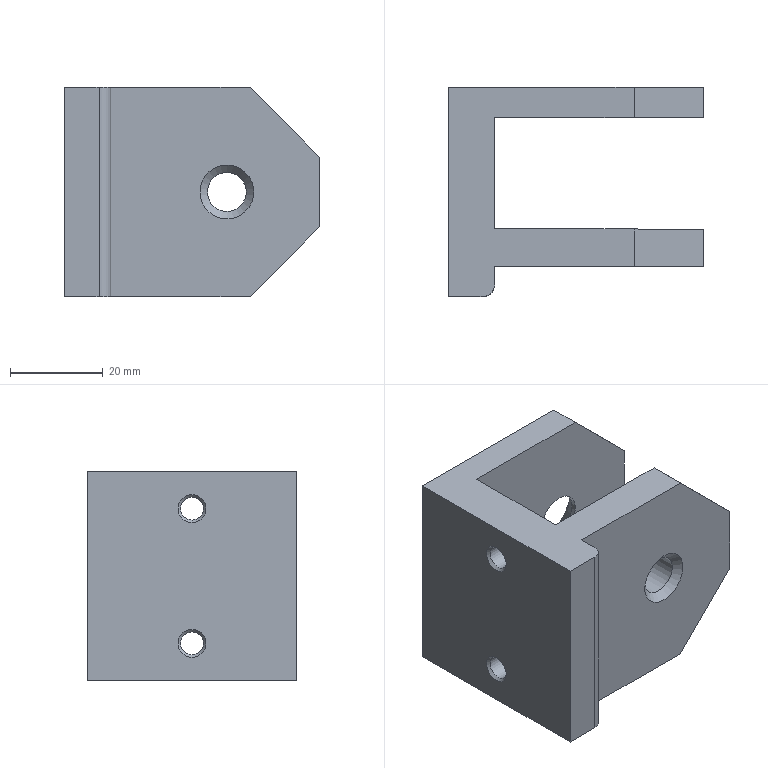Part | STEP file | HBLTBBN45_b | 1 solid | 26 faces | box 55 x 45 x 45 mm | volume 44256 mm3 | plane 16 | cylinder 5 | cone 5 | commonest cylinder face diameters 4.917 x2 5 x1 8.376 x1 10 x1
STEP:
#1=CARTESIAN_POINT('',(55.,45.,7.5));
#2=VERTEX_POINT('',#1);
#3=CARTESIAN_POINT('',(40.,45.,22.5));
#4=VERTEX_POINT('',#3);
#5=CARTESIAN_POINT('',(55.,45.,7.5));
#6=DIRECTION('',(-0.7071,0.,0.7071));
#7=VECTOR('',#6,1000.);
#8=LINE('',#5,#7);
#9=EDGE_CURVE('',#2,#4,#8,.T.);
#10=ORIENTED_EDGE('',*,*,#9,.F.);
#11=CARTESIAN_POINT('',(55.,45.,-7.5));
#12=VERTEX_POINT('',#11);
#13=CARTESIAN_POINT('',(55.,45.,22.5));
#14=DIRECTION('',(0.,0.,-1.));
#15=VECTOR('',#14,1000.);
#16=LINE('',#13,#15);
#17=EDGE_CURVE('',#2,#12,#16,.T.);
#18=ORIENTED_EDGE('',*,*,#17,.T.);
#19=CARTESIAN_POINT('',(40.,45.,-22.5));
#20=VERTEX_POINT('',#19);
#21=CARTESIAN_POINT('',(40.,45.,-22.5));
#22=DIRECTION('',(0.7071,0.,0.7071));
#23=VECTOR('',#22,1000.);
#24=LINE('',#21,#23);
#25=EDGE_CURVE('',#20,#12,#24,.T.);
#26=ORIENTED_EDGE('',*,*,#25,.F.);
#27=CARTESIAN_POINT('',(0.,45.,-22.5));
#28=VERTEX_POINT('',#27);
#29=CARTESIAN_POINT('',(55.,45.,-22.5));
#30=DIRECTION('',(-1.,0.,0.));
#31=VECTOR('',#30,1000.);
#32=LINE('',#29,#31);
#33=EDGE_CURVE('',#20,#28,#32,.T.);
#34=ORIENTED_EDGE('',*,*,#33,.T.);
#35=CARTESIAN_POINT('',(0.,45.,22.5));
#36=VERTEX_POINT('',#35);
#37=CARTESIAN_POINT('',(0.,45.,22.5));
#38=DIRECTION('',(0.,0.,-1.));
#39=VECTOR('',#38,1000.);
#40=LINE('',#37,#39);
#41=EDGE_CURVE('',#36,#28,#40,.T.);
#42=ORIENTED_EDGE('',*,*,#41,.F.);
#43=CARTESIAN_POINT('',(55.,45.,22.5));
#44=DIRECTION('',(-1.,0.,0.));
#45=VECTOR('',#44,1000.);
#46=LINE('',#43,#45);
#47=EDGE_CURVE('',#4,#36,#46,.T.);
#48=ORIENTED_EDGE('',*,*,#47,.F.);
#49=EDGE_LOOP('',(#10,#18,#26,#34,#42,#48));
#50=FACE_OUTER_BOUND('',#49,.T.);
#51=CARTESIAN_POINT('',(35.,45.,-10.5));
#52=VERTEX_POINT('',#51);
#53=CARTESIAN_POINT('',(35.,45.,0.));
#54=DIRECTION('',(0.,-1.,0.));
#55=DIRECTION('',(0.,0.,-1.));
#56=AXIS2_PLACEMENT_3D('',#53,#54,#55);
#57=CIRCLE('',#56,10.5);
#58=EDGE_CURVE('',#52,#52,#57,.T.);
#59=ORIENTED_EDGE('',*,*,#58,.T.);
#60=EDGE_LOOP('',(#59));
#61=FACE_BOUND('',#60,.T.);
#62=CARTESIAN_POINT('',(55.,45.,22.5));
#63=DIRECTION('',(0.,-1.,0.));
#64=DIRECTION('',(0.,0.,-1.));
#65=AXIS2_PLACEMENT_3D('',#62,#63,#64);
#66=PLANE('',#65);
#67=ADVANCED_FACE('',(#50,#61),#66,.F.);
#68=CARTESIAN_POINT('',(40.,6.5,22.5));
#69=VERTEX_POINT('',#68);
#70=CARTESIAN_POINT('',(55.,6.5,7.5));
#71=VERTEX_POINT('',#70);
#72=CARTESIAN_POINT('',(25.,6.5,37.5));
#73=DIRECTION('',(0.7071,0.,-0.7071));
#74=VECTOR('',#73,1000.);
#75=LINE('',#72,#74);
#76=EDGE_CURVE('',#69,#71,#75,.T.);
#77=ORIENTED_EDGE('',*,*,#76,.F.);
#78=CARTESIAN_POINT('',(10.,6.5,22.5));
#79=VERTEX_POINT('',#78);
#80=CARTESIAN_POINT('',(10.,6.5,22.5));
#81=DIRECTION('',(1.,0.,0.));
#82=VECTOR('',#81,1000.);
#83=LINE('',#80,#82);
#84=EDGE_CURVE('',#79,#69,#83,.T.);
#85=ORIENTED_EDGE('',*,*,#84,.F.);
#86=CARTESIAN_POINT('',(10.,6.5,-22.5));
#87=VERTEX_POINT('',#86);
#88=CARTESIAN_POINT('',(10.,6.5,22.5));
#89=DIRECTION('',(0.,0.,-1.));
#90=VECTOR('',#89,1000.);
#91=LINE('',#88,#90);
#92=EDGE_CURVE('',#79,#87,#91,.T.);
#93=ORIENTED_EDGE('',*,*,#92,.T.);
#94=CARTESIAN_POINT('',(40.,6.5,-22.5));
#95=VERTEX_POINT('',#94);
#96=CARTESIAN_POINT('',(10.,6.5,-22.5));
#97=DIRECTION('',(1.,0.,0.));
#98=VECTOR('',#97,1000.);
#99=LINE('',#96,#98);
#100=EDGE_CURVE('',#87,#95,#99,.T.);
#101=ORIENTED_EDGE('',*,*,#100,.T.);
#102=CARTESIAN_POINT('',(55.,6.5,-7.5));
#103=VERTEX_POINT('',#102);
#104=CARTESIAN_POINT('',(47.5,6.5,-15.));
#105=DIRECTION('',(-0.7071,0.,-0.7071));
#106=VECTOR('',#105,1000.);
#107=LINE('',#104,#106);
#108=EDGE_CURVE('',#103,#95,#107,.T.);
#109=ORIENTED_EDGE('',*,*,#108,.F.);
#110=CARTESIAN_POINT('',(55.,6.5,22.5));
#111=DIRECTION('',(0.,0.,-1.));
#112=VECTOR('',#111,1000.);
#113=LINE('',#110,#112);
#114=EDGE_CURVE('',#71,#103,#113,.T.);
#115=ORIENTED_EDGE('',*,*,#114,.F.);
#116=EDGE_LOOP('',(#77,#85,#93,#101,#109,#115));
#117=FACE_OUTER_BOUND('',#116,.T.);
#118=CARTESIAN_POINT('',(35.,6.5,-5.8));
#119=VERTEX_POINT('',#118);
#120=CARTESIAN_POINT('',(35.,6.5,5.8));
#121=VERTEX_POINT('',#120);
#122=CARTESIAN_POINT('',(35.,6.5,0.));
#123=DIRECTION('',(0.,-1.,0.));
#124=DIRECTION('',(0.,0.,-1.));
#125=AXIS2_PLACEMENT_3D('',#122,#123,#124);
#126=CIRCLE('',#125,5.8);
#127=EDGE_CURVE('',#119,#121,#126,.T.);
#128=ORIENTED_EDGE('',*,*,#127,.F.);
#129=CARTESIAN_POINT('',(35.,6.5,0.));
#130=DIRECTION('',(0.,-1.,0.));
#131=DIRECTION('',(0.,0.,-1.));
#132=AXIS2_PLACEMENT_3D('',#129,#130,#131);
#133=CIRCLE('',#132,5.8);
#134=EDGE_CURVE('',#121,#119,#133,.T.);
#135=ORIENTED_EDGE('',*,*,#134,.F.);
#136=EDGE_LOOP('',(#128,#135));
#137=FACE_BOUND('',#136,.T.);
#138=CARTESIAN_POINT('',(10.,6.5,22.5));
#139=DIRECTION('',(0.,1.,0.));
#140=DIRECTION('',(-1.,0.,0.));
#141=AXIS2_PLACEMENT_3D('',#138,#139,#140);
#142=PLANE('',#141);
#143=ADVANCED_FACE('',(#117,#137),#142,.F.);
#144=CARTESIAN_POINT('',(55.,14.5,7.5));
#145=VERTEX_POINT('',#144);
#146=CARTESIAN_POINT('',(55.,45.,7.5));
#147=DIRECTION('',(0.,-1.,0.));
#148=VECTOR('',#147,1000.);
#149=LINE('',#146,#148);
#150=EDGE_CURVE('',#145,#71,#149,.T.);
#151=ORIENTED_EDGE('',*,*,#150,.T.);
#152=ORIENTED_EDGE('',*,*,#114,.T.);
#153=CARTESIAN_POINT('',(55.,14.5,-7.5));
#154=VERTEX_POINT('',#153);
#155=CARTESIAN_POINT('',(55.,45.,-7.5));
#156=DIRECTION('',(0.,-1.,0.));
#157=VECTOR('',#156,1000.);
#158=LINE('',#155,#157);
#159=EDGE_CURVE('',#154,#103,#158,.T.);
#160=ORIENTED_EDGE('',*,*,#159,.F.);
#161=CARTESIAN_POINT('',(55.,14.5,22.5));
#162=DIRECTION('',(0.,0.,-1.));
#163=VECTOR('',#162,1000.);
#164=LINE('',#161,#163);
#165=EDGE_CURVE('',#145,#154,#164,.T.);
#166=ORIENTED_EDGE('',*,*,#165,.F.);
#167=EDGE_LOOP('',(#151,#152,#160,#166));
#168=FACE_OUTER_BOUND('',#167,.T.);
#169=CARTESIAN_POINT('',(55.,6.5,22.5));
#170=DIRECTION('',(-1.,0.,0.));
#171=DIRECTION('',(0.,0.,1.));
#172=AXIS2_PLACEMENT_3D('',#169,#170,#171);
#173=PLANE('',#172);
#174=ADVANCED_FACE('',(#168),#173,.F.);
#175=CARTESIAN_POINT('',(40.,14.5,22.5));
#176=VERTEX_POINT('',#175);
#177=CARTESIAN_POINT('',(47.5,14.5,15.));
#178=DIRECTION('',(-0.7071,0.,0.7071));
#179=VECTOR('',#178,1000.);
#180=LINE('',#177,#179);
#181=EDGE_CURVE('',#145,#176,#180,.T.);
#182=ORIENTED_EDGE('',*,*,#181,.F.);
#183=ORIENTED_EDGE('',*,*,#165,.T.);
#184=CARTESIAN_POINT('',(40.,14.5,-22.5));
#185=VERTEX_POINT('',#184);
#186=CARTESIAN_POINT('',(70.,14.5,7.5));
#187=DIRECTION('',(0.7071,0.,0.7071));
#188=VECTOR('',#187,1000.);
#189=LINE('',#186,#188);
#190=EDGE_CURVE('',#185,#154,#189,.T.);
#191=ORIENTED_EDGE('',*,*,#190,.F.);
#192=CARTESIAN_POINT('',(10.,14.5,-22.5));
#193=VERTEX_POINT('',#192);
#194=CARTESIAN_POINT('',(55.,14.5,-22.5));
#195=DIRECTION('',(-1.,0.,0.));
#196=VECTOR('',#195,1000.);
#197=LINE('',#194,#196);
#198=EDGE_CURVE('',#185,#193,#197,.T.);
#199=ORIENTED_EDGE('',*,*,#198,.T.);
#200=CARTESIAN_POINT('',(10.,14.5,22.5));
#201=VERTEX_POINT('',#200);
#202=CARTESIAN_POINT('',(10.,14.5,22.5));
#203=DIRECTION('',(0.,0.,-1.));
#204=VECTOR('',#203,1000.);
#205=LINE('',#202,#204);
#206=EDGE_CURVE('',#201,#193,#205,.T.);
#207=ORIENTED_EDGE('',*,*,#206,.F.);
#208=CARTESIAN_POINT('',(55.,14.5,22.5));
#209=DIRECTION('',(-1.,0.,0.));
#210=VECTOR('',#209,1000.);
#211=LINE('',#208,#210);
#212=EDGE_CURVE('',#176,#201,#211,.T.);
#213=ORIENTED_EDGE('',*,*,#212,.F.);
#214=EDGE_LOOP('',(#182,#183,#191,#199,#207,#213));
#215=FACE_OUTER_BOUND('',#214,.T.);
#216=CARTESIAN_POINT('',(35.,14.5,-5.));
#217=VERTEX_POINT('',#216);
#218=CARTESIAN_POINT('',(35.,14.5,0.));
#219=DIRECTION('',(0.,-1.,0.));
#220=DIRECTION('',(0.,0.,-1.));
#221=AXIS2_PLACEMENT_3D('',#218,#219,#220);
#222=CIRCLE('',#221,5.);
#223=EDGE_CURVE('',#217,#217,#222,.T.);
#224=ORIENTED_EDGE('',*,*,#223,.T.);
#225=EDGE_LOOP('',(#224));
#226=FACE_BOUND('',#225,.T.);
#227=CARTESIAN_POINT('',(55.,14.5,22.5));
#228=DIRECTION('',(0.,-1.,0.));
#229=DIRECTION('',(0.,0.,-1.));
#230=AXIS2_PLACEMENT_3D('',#227,#228,#229);
#231=PLANE('',#230);
#232=ADVANCED_FACE('',(#215,#226),#231,.F.);
#233=CARTESIAN_POINT('',(40.,38.5,22.5));
#234=VERTEX_POINT('',#233);
#235=CARTESIAN_POINT('',(55.,38.5,7.5));
#236=VERTEX_POINT('',#235);
#237=CARTESIAN_POINT('',(25.,38.5,37.5));
#238=DIRECTION('',(0.7071,0.,-0.7071));
#239=VECTOR('',#238,1000.);
#240=LINE('',#237,#239);
#241=EDGE_CURVE('',#234,#236,#240,.T.);
#242=ORIENTED_EDGE('',*,*,#241,.F.);
#243=CARTESIAN_POINT('',(10.,38.5,22.5));
#244=VERTEX_POINT('',#243);
#245=CARTESIAN_POINT('',(10.,38.5,22.5));
#246=DIRECTION('',(1.,0.,0.));
#247=VECTOR('',#246,1000.);
#248=LINE('',#245,#247);
#249=EDGE_CURVE('',#244,#234,#248,.T.);
#250=ORIENTED_EDGE('',*,*,#249,.F.);
#251=CARTESIAN_POINT('',(10.,38.5,-22.5));
#252=VERTEX_POINT('',#251);
#253=CARTESIAN_POINT('',(10.,38.5,22.5));
#254=DIRECTION('',(0.,0.,-1.));
#255=VECTOR('',#254,1000.);
#256=LINE('',#253,#255);
#257=EDGE_CURVE('',#244,#252,#256,.T.);
#258=ORIENTED_EDGE('',*,*,#257,.T.);
#259=CARTESIAN_POINT('',(40.,38.5,-22.5));
#260=VERTEX_POINT('',#259);
#261=CARTESIAN_POINT('',(10.,38.5,-22.5));
#262=DIRECTION('',(1.,0.,0.));
#263=VECTOR('',#262,1000.);
#264=LINE('',#261,#263);
#265=EDGE_CURVE('',#252,#260,#264,.T.);
#266=ORIENTED_EDGE('',*,*,#265,.T.);
#267=CARTESIAN_POINT('',(55.,38.5,-7.5));
#268=VERTEX_POINT('',#267);
#269=CARTESIAN_POINT('',(47.5,38.5,-15.));
#270=DIRECTION('',(-0.7071,0.,-0.7071));
#271=VECTOR('',#270,1000.);
#272=LINE('',#269,#271);
#273=EDGE_CURVE('',#268,#260,#272,.T.);
#274=ORIENTED_EDGE('',*,*,#273,.F.);
#275=CARTESIAN_POINT('',(55.,38.5,22.5));
#276=DIRECTION('',(0.,0.,-1.));
#277=VECTOR('',#276,1000.);
#278=LINE('',#275,#277);
#279=EDGE_CURVE('',#236,#268,#278,.T.);
#280=ORIENTED_EDGE('',*,*,#279,.F.);
#281=EDGE_LOOP('',(#242,#250,#258,#266,#274,#280));
#282=FACE_OUTER_BOUND('',#281,.T.);
#283=CARTESIAN_POINT('',(35.,38.5,-5.));
#284=VERTEX_POINT('',#283);
#285=CARTESIAN_POINT('',(35.,38.5,5.));
#286=VERTEX_POINT('',#285);
#287=CARTESIAN_POINT('',(35.,38.5,0.));
#288=DIRECTION('',(0.,-1.,0.));
#289=DIRECTION('',(0.,0.,-1.));
#290=AXIS2_PLACEMENT_3D('',#287,#288,#289);
#291=CIRCLE('',#290,5.);
#292=EDGE_CURVE('',#284,#286,#291,.T.);
#293=ORIENTED_EDGE('',*,*,#292,.F.);
#294=CARTESIAN_POINT('',(35.,38.5,0.));
#295=DIRECTION('',(0.,-1.,0.));
#296=DIRECTION('',(0.,0.,-1.));
#297=AXIS2_PLACEMENT_3D('',#294,#295,#296);
#298=CIRCLE('',#297,5.);
#299=EDGE_CURVE('',#286,#284,#298,.T.);
#300=ORIENTED_EDGE('',*,*,#299,.F.);
#301=EDGE_LOOP('',(#293,#300));
#302=FACE_BOUND('',#301,.T.);
#303=CARTESIAN_POINT('',(10.,38.5,22.5));
#304=DIRECTION('',(0.,1.,0.));
#305=DIRECTION('',(0.,0.,1.));
#306=AXIS2_PLACEMENT_3D('',#303,#304,#305);
#307=PLANE('',#306);
#308=ADVANCED_FACE('',(#282,#302),#307,.F.);
#309=CARTESIAN_POINT('',(55.,45.,7.5));
#310=DIRECTION('',(0.,-1.,0.));
#311=VECTOR('',#310,1000.);
#312=LINE('',#309,#311);
#313=EDGE_CURVE('',#2,#236,#312,.T.);
#314=ORIENTED_EDGE('',*,*,#313,.T.);
#315=ORIENTED_EDGE('',*,*,#279,.T.);
#316=CARTESIAN_POINT('',(55.,45.,-7.5));
#317=DIRECTION('',(0.,-1.,0.));
#318=VECTOR('',#317,1000.);
#319=LINE('',#316,#318);
#320=EDGE_CURVE('',#12,#268,#319,.T.);
#321=ORIENTED_EDGE('',*,*,#320,.F.);
#322=ORIENTED_EDGE('',*,*,#17,.F.);
#323=EDGE_LOOP('',(#314,#315,#321,#322));
#324=FACE_OUTER_BOUND('',#323,.T.);
#325=CARTESIAN_POINT('',(55.,38.5,22.5));
#326=DIRECTION('',(-1.,0.,0.));
#327=DIRECTION('',(0.,0.,1.));
#328=AXIS2_PLACEMENT_3D('',#325,#326,#327);
#329=PLANE('',#328);
#330=ADVANCED_FACE('',(#324),#329,.F.);
#331=ORIENTED_EDGE('',*,*,#84,.T.);
#332=CARTESIAN_POINT('',(40.,2.5,22.5));
#333=DIRECTION('',(0.,1.,0.));
#334=VECTOR('',#333,1000.);
#335=LINE('',#332,#334);
#336=EDGE_CURVE('',#69,#176,#335,.T.);
#337=ORIENTED_EDGE('',*,*,#336,.T.);
#338=ORIENTED_EDGE('',*,*,#212,.T.);
#339=CARTESIAN_POINT('',(10.,14.5,22.5));
#340=DIRECTION('',(0.,1.,0.));
#341=VECTOR('',#340,1000.);
#342=LINE('',#339,#341);
#343=EDGE_CURVE('',#201,#244,#342,.T.);
#344=ORIENTED_EDGE('',*,*,#343,.T.);
#345=ORIENTED_EDGE('',*,*,#249,.T.);
#346=CARTESIAN_POINT('',(40.,45.,22.5));
#347=DIRECTION('',(0.,-1.,0.));
#348=VECTOR('',#347,1000.);
#349=LINE('',#346,#348);
#350=EDGE_CURVE('',#4,#234,#349,.T.);
#351=ORIENTED_EDGE('',*,*,#350,.F.);
#352=ORIENTED_EDGE('',*,*,#47,.T.);
#353=CARTESIAN_POINT('',(0.,0.,22.5));
#354=VERTEX_POINT('',#353);
#355=CARTESIAN_POINT('',(0.,45.,22.5));
#356=DIRECTION('',(0.,-1.,0.));
#357=VECTOR('',#356,1000.);
#358=LINE('',#355,#357);
#359=EDGE_CURVE('',#36,#354,#358,.T.);
#360=ORIENTED_EDGE('',*,*,#359,.T.);
#361=CARTESIAN_POINT('',(7.5,0.,22.5));
#362=VERTEX_POINT('',#361);
#363=CARTESIAN_POINT('',(0.,0.,22.5));
#364=DIRECTION('',(1.,0.,0.));
#365=VECTOR('',#364,1000.);
#366=LINE('',#363,#365);
#367=EDGE_CURVE('',#354,#362,#366,.T.);
#368=ORIENTED_EDGE('',*,*,#367,.T.);
#369=CARTESIAN_POINT('',(10.,2.5,22.5));
#370=VERTEX_POINT('',#369);
#371=CARTESIAN_POINT('',(7.5,2.5,22.5));
#372=DIRECTION('',(0.,0.,1.));
#373=DIRECTION('',(1.,0.,0.));
#374=AXIS2_PLACEMENT_3D('',#371,#372,#373);
#375=CIRCLE('',#374,2.5);
#376=EDGE_CURVE('',#362,#370,#375,.T.);
#377=ORIENTED_EDGE('',*,*,#376,.T.);
#378=CARTESIAN_POINT('',(10.,2.5,22.5));
#379=DIRECTION('',(0.,1.,0.));
#380=VECTOR('',#379,1000.);
#381=LINE('',#378,#380);
#382=EDGE_CURVE('',#370,#79,#381,.T.);
#383=ORIENTED_EDGE('',*,*,#382,.T.);
#384=EDGE_LOOP('',(#331,#337,#338,#344,#345,#351,#352,#360,#368,#377,#383));
#385=FACE_OUTER_BOUND('',#384,.T.);
#386=CARTESIAN_POINT('',(7.5,2.5,22.5));
#387=DIRECTION('',(0.,0.,1.));
#388=DIRECTION('',(1.,0.,0.));
#389=AXIS2_PLACEMENT_3D('',#386,#387,#388);
#390=PLANE('',#389);
#391=ADVANCED_FACE('',(#385),#390,.T.);
#392=CARTESIAN_POINT('',(40.,2.5,-22.5));
#393=DIRECTION('',(0.,1.,0.));
#394=VECTOR('',#393,1000.);
#395=LINE('',#392,#394);
#396=EDGE_CURVE('',#95,#185,#395,.T.);
#397=ORIENTED_EDGE('',*,*,#396,.F.);
#398=ORIENTED_EDGE('',*,*,#100,.F.);
#399=CARTESIAN_POINT('',(10.,2.5,-22.5));
#400=VERTEX_POINT('',#399);
#401=CARTESIAN_POINT('',(10.,2.5,-22.5));
#402=DIRECTION('',(0.,1.,0.));
#403=VECTOR('',#402,1000.);
#404=LINE('',#401,#403);
#405=EDGE_CURVE('',#400,#87,#404,.T.);
#406=ORIENTED_EDGE('',*,*,#405,.F.);
#407=CARTESIAN_POINT('',(7.5,0.,-22.5));
#408=VERTEX_POINT('',#407);
#409=CARTESIAN_POINT('',(7.5,2.5,-22.5));
#410=DIRECTION('',(0.,0.,1.));
#411=DIRECTION('',(1.,0.,0.));
#412=AXIS2_PLACEMENT_3D('',#409,#410,#411);
#413=CIRCLE('',#412,2.5);
#414=EDGE_CURVE('',#408,#400,#413,.T.);
#415=ORIENTED_EDGE('',*,*,#414,.F.);
#416=CARTESIAN_POINT('',(0.,0.,-22.5));
#417=VERTEX_POINT('',#416);
#418=CARTESIAN_POINT('',(0.,0.,-22.5));
#419=DIRECTION('',(1.,0.,0.));
#420=VECTOR('',#419,1000.);
#421=LINE('',#418,#420);
#422=EDGE_CURVE('',#417,#408,#421,.T.);
#423=ORIENTED_EDGE('',*,*,#422,.F.);
#424=CARTESIAN_POINT('',(0.,45.,-22.5));
#425=DIRECTION('',(0.,-1.,0.));
#426=VECTOR('',#425,1000.);
#427=LINE('',#424,#426);
#428=EDGE_CURVE('',#28,#417,#427,.T.);
#429=ORIENTED_EDGE('',*,*,#428,.F.);
#430=ORIENTED_EDGE('',*,*,#33,.F.);
#431=CARTESIAN_POINT('',(40.,45.,-22.5));
#432=DIRECTION('',(0.,-1.,0.));
#433=VECTOR('',#432,1000.);
#434=LINE('',#431,#433);
#435=EDGE_CURVE('',#20,#260,#434,.T.);
#436=ORIENTED_EDGE('',*,*,#435,.T.);
#437=ORIENTED_EDGE('',*,*,#265,.F.);
#438=CARTESIAN_POINT('',(10.,14.5,-22.5));
#439=DIRECTION('',(0.,1.,0.));
#440=VECTOR('',#439,1000.);
#441=LINE('',#438,#440);
#442=EDGE_CURVE('',#193,#252,#441,.T.);
#443=ORIENTED_EDGE('',*,*,#442,.F.);
#444=ORIENTED_EDGE('',*,*,#198,.F.);
#445=EDGE_LOOP('',(#397,#398,#406,#415,#423,#429,#430,#436,#437,#443,#444));
#446=FACE_OUTER_BOUND('',#445,.T.);
#447=CARTESIAN_POINT('',(7.5,2.5,-22.5));
#448=DIRECTION('',(0.,0.,1.));
#449=DIRECTION('',(1.,0.,0.));
#450=AXIS2_PLACEMENT_3D('',#447,#448,#449);
#451=PLANE('',#450);
#452=ADVANCED_FACE('',(#446),#451,.F.);
#453=ORIENTED_EDGE('',*,*,#428,.T.);
#454=CARTESIAN_POINT('',(0.,0.,22.5));
#455=DIRECTION('',(0.,0.,-1.));
#456=VECTOR('',#455,1000.);
#457=LINE('',#454,#456);
#458=EDGE_CURVE('',#354,#417,#457,.T.);
#459=ORIENTED_EDGE('',*,*,#458,.F.);
#460=ORIENTED_EDGE('',*,*,#359,.F.);
#461=ORIENTED_EDGE('',*,*,#41,.T.);
#462=EDGE_LOOP('',(#453,#459,#460,#461));
#463=FACE_OUTER_BOUND('',#462,.T.);
#464=CARTESIAN_POINT('',(0.,22.5,-17.5));
#465=VERTEX_POINT('',#464);
#466=CARTESIAN_POINT('',(0.,22.5,-14.5));
#467=DIRECTION('',(1.,0.,0.));
#468=DIRECTION('',(0.,0.,-1.));
#469=AXIS2_PLACEMENT_3D('',#466,#467,#468);
#470=CIRCLE('',#469,3.);
#471=EDGE_CURVE('',#465,#465,#470,.T.);
#472=ORIENTED_EDGE('',*,*,#471,.T.);
#473=EDGE_LOOP('',(#472));
#474=FACE_BOUND('',#473,.T.);
#475=CARTESIAN_POINT('',(0.,22.5,11.5));
#476=VERTEX_POINT('',#475);
#477=CARTESIAN_POINT('',(0.,22.5,14.5));
#478=DIRECTION('',(1.,0.,0.));
#479=DIRECTION('',(0.,0.,-1.));
#480=AXIS2_PLACEMENT_3D('',#477,#478,#479);
#481=CIRCLE('',#480,3.);
#482=EDGE_CURVE('',#476,#476,#481,.T.);
#483=ORIENTED_EDGE('',*,*,#482,.T.);
#484=EDGE_LOOP('',(#483));
#485=FACE_BOUND('',#484,.T.);
#486=CARTESIAN_POINT('',(0.,45.,22.5));
#487=DIRECTION('',(1.,0.,0.));
#488=DIRECTION('',(0.,0.,-1.));
#489=AXIS2_PLACEMENT_3D('',#486,#487,#488);
#490=PLANE('',#489);
#491=ADVANCED_FACE('',(#463,#474,#485),#490,.F.);
#492=ORIENTED_EDGE('',*,*,#422,.T.);
#493=CARTESIAN_POINT('',(7.5,0.,22.5));
#494=DIRECTION('',(0.,0.,-1.));
#495=VECTOR('',#494,1000.);
#496=LINE('',#493,#495);
#497=EDGE_CURVE('',#362,#408,#496,.T.);
#498=ORIENTED_EDGE('',*,*,#497,.F.);
#499=ORIENTED_EDGE('',*,*,#367,.F.);
#500=ORIENTED_EDGE('',*,*,#458,.T.);
#501=EDGE_LOOP('',(#492,#498,#499,#500));
#502=FACE_OUTER_BOUND('',#501,.T.);
#503=CARTESIAN_POINT('',(0.,0.,22.5));
#504=DIRECTION('',(0.,1.,0.));
#505=DIRECTION('',(0.,0.,1.));
#506=AXIS2_PLACEMENT_3D('',#503,#504,#505);
#507=PLANE('',#506);
#508=ADVANCED_FACE('',(#502),#507,.F.);
#509=ORIENTED_EDGE('',*,*,#414,.T.);
#510=CARTESIAN_POINT('',(10.,2.5,22.5));
#511=DIRECTION('',(0.,0.,-1.));
#512=VECTOR('',#511,1000.);
#513=LINE('',#510,#512);
#514=EDGE_CURVE('',#370,#400,#513,.T.);
#515=ORIENTED_EDGE('',*,*,#514,.F.);
#516=ORIENTED_EDGE('',*,*,#376,.F.);
#517=ORIENTED_EDGE('',*,*,#497,.T.);
#518=EDGE_LOOP('',(#509,#515,#516,#517));
#519=FACE_OUTER_BOUND('',#518,.T.);
#520=CARTESIAN_POINT('',(7.5,2.5,22.5));
#521=DIRECTION('',(0.,0.,-1.));
#522=DIRECTION('',(-1.,0.,0.));
#523=AXIS2_PLACEMENT_3D('',#520,#521,#522);
#524=CYLINDRICAL_SURFACE('',#523,2.5);
#525=ADVANCED_FACE('',(#519),#524,.T.);
#526=ORIENTED_EDGE('',*,*,#405,.T.);
#527=ORIENTED_EDGE('',*,*,#92,.F.);
#528=ORIENTED_EDGE('',*,*,#382,.F.);
#529=ORIENTED_EDGE('',*,*,#514,.T.);
#530=EDGE_LOOP('',(#526,#527,#528,#529));
#531=FACE_OUTER_BOUND('',#530,.T.);
#532=CARTESIAN_POINT('',(10.,2.5,22.5));
#533=DIRECTION('',(-1.,0.,0.));
#534=DIRECTION('',(0.,0.,1.));
#535=AXIS2_PLACEMENT_3D('',#532,#533,#534);
#536=PLANE('',#535);
#537=ADVANCED_FACE('',(#531),#536,.F.);
#538=ORIENTED_EDGE('',*,*,#442,.T.);
#539=ORIENTED_EDGE('',*,*,#257,.F.);
#540=ORIENTED_EDGE('',*,*,#343,.F.);
#541=ORIENTED_EDGE('',*,*,#206,.T.);
#542=EDGE_LOOP('',(#538,#539,#540,#541));
#543=FACE_OUTER_BOUND('',#542,.T.);
#544=CARTESIAN_POINT('',(10.,22.5,-16.959));
#545=VERTEX_POINT('',#544);
#546=CARTESIAN_POINT('',(10.,22.5,-12.041));
#547=VERTEX_POINT('',#546);
#548=CARTESIAN_POINT('',(10.,22.5,-14.5));
#549=DIRECTION('',(1.,0.,0.));
#550=DIRECTION('',(0.,0.,-1.));
#551=AXIS2_PLACEMENT_3D('',#548,#549,#550);
#552=CIRCLE('',#551,2.458);
#553=EDGE_CURVE('',#545,#547,#552,.T.);
#554=ORIENTED_EDGE('',*,*,#553,.F.);
#555=CARTESIAN_POINT('',(10.,22.5,-14.5));
#556=DIRECTION('',(1.,0.,0.));
#557=DIRECTION('',(0.,0.,-1.));
#558=AXIS2_PLACEMENT_3D('',#555,#556,#557);
#559=CIRCLE('',#558,2.458);
#560=EDGE_CURVE('',#547,#545,#559,.T.);
#561=ORIENTED_EDGE('',*,*,#560,.F.);
#562=EDGE_LOOP('',(#554,#561));
#563=FACE_BOUND('',#562,.T.);
#564=CARTESIAN_POINT('',(10.,22.5,12.041));
#565=VERTEX_POINT('',#564);
#566=CARTESIAN_POINT('',(10.,22.5,16.959));
#567=VERTEX_POINT('',#566);
#568=CARTESIAN_POINT('',(10.,22.5,14.5));
#569=DIRECTION('',(1.,0.,0.));
#570=DIRECTION('',(0.,0.,-1.));
#571=AXIS2_PLACEMENT_3D('',#568,#569,#570);
#572=CIRCLE('',#571,2.458);
#573=EDGE_CURVE('',#565,#567,#572,.T.);
#574=ORIENTED_EDGE('',*,*,#573,.F.);
#575=CARTESIAN_POINT('',(10.,22.5,14.5));
#576=DIRECTION('',(1.,0.,0.));
#577=DIRECTION('',(0.,0.,-1.));
#578=AXIS2_PLACEMENT_3D('',#575,#576,#577);
#579=CIRCLE('',#578,2.458);
#580=EDGE_CURVE('',#567,#565,#579,.T.);
#581=ORIENTED_EDGE('',*,*,#580,.F.);
#582=EDGE_LOOP('',(#574,#581));
#583=FACE_BOUND('',#582,.T.);
#584=CARTESIAN_POINT('',(10.,14.5,22.5));
#585=DIRECTION('',(-1.,0.,0.));
#586=DIRECTION('',(0.,0.,1.));
#587=AXIS2_PLACEMENT_3D('',#584,#585,#586);
#588=PLANE('',#587);
#589=ADVANCED_FACE('',(#543,#563,#583),#588,.F.);
#590=ORIENTED_EDGE('',*,*,#273,.T.);
#591=ORIENTED_EDGE('',*,*,#435,.F.);
#592=ORIENTED_EDGE('',*,*,#25,.T.);
#593=ORIENTED_EDGE('',*,*,#320,.T.);
#594=EDGE_LOOP('',(#590,#591,#592,#593));
#595=FACE_OUTER_BOUND('',#594,.T.);
#596=CARTESIAN_POINT('',(40.,45.,-22.5));
#597=DIRECTION('',(0.7071,0.,-0.7071));
#598=DIRECTION('',(-0.7071,0.,-0.7071));
#599=AXIS2_PLACEMENT_3D('',#596,#597,#598);
#600=PLANE('',#599);
#601=ADVANCED_FACE('',(#595),#600,.T.);
#602=ORIENTED_EDGE('',*,*,#108,.T.);
#603=ORIENTED_EDGE('',*,*,#396,.T.);
#604=ORIENTED_EDGE('',*,*,#190,.T.);
#605=ORIENTED_EDGE('',*,*,#159,.T.);
#606=EDGE_LOOP('',(#602,#603,#604,#605));
#607=FACE_OUTER_BOUND('',#606,.T.);
#608=CARTESIAN_POINT('',(40.,45.,-22.5));
#609=DIRECTION('',(0.7071,0.,-0.7071));
#610=DIRECTION('',(-0.7071,0.,-0.7071));
#611=AXIS2_PLACEMENT_3D('',#608,#609,#610);
#612=PLANE('',#611);
#613=ADVANCED_FACE('',(#607),#612,.T.);
#614=ORIENTED_EDGE('',*,*,#241,.T.);
#615=ORIENTED_EDGE('',*,*,#313,.F.);
#616=ORIENTED_EDGE('',*,*,#9,.T.);
#617=ORIENTED_EDGE('',*,*,#350,.T.);
#618=EDGE_LOOP('',(#614,#615,#616,#617));
#619=FACE_OUTER_BOUND('',#618,.T.);
#620=CARTESIAN_POINT('',(55.,45.,7.5));
#621=DIRECTION('',(0.7071,0.,0.7071));
#622=DIRECTION('',(0.7071,0.,-0.7071));
#623=AXIS2_PLACEMENT_3D('',#620,#621,#622);
#624=PLANE('',#623);
#625=ADVANCED_FACE('',(#619),#624,.T.);
#626=ORIENTED_EDGE('',*,*,#76,.T.);
#627=ORIENTED_EDGE('',*,*,#150,.F.);
#628=ORIENTED_EDGE('',*,*,#181,.T.);
#629=ORIENTED_EDGE('',*,*,#336,.F.);
#630=EDGE_LOOP('',(#626,#627,#628,#629));
#631=FACE_OUTER_BOUND('',#630,.T.);
#632=CARTESIAN_POINT('',(55.,45.,7.5));
#633=DIRECTION('',(0.7071,0.,0.7071));
#634=DIRECTION('',(0.7071,0.,-0.7071));
#635=AXIS2_PLACEMENT_3D('',#632,#633,#634);
#636=PLANE('',#635);
#637=ADVANCED_FACE('',(#631),#636,.T.);
#638=CARTESIAN_POINT('',(35.,13.688,-4.188));
#639=VERTEX_POINT('',#638);
#640=CARTESIAN_POINT('',(35.,13.688,4.188));
#641=VERTEX_POINT('',#640);
#642=CARTESIAN_POINT('',(35.,13.688,0.));
#643=DIRECTION('',(0.,-1.,0.));
#644=DIRECTION('',(0.,0.,-1.));
#645=AXIS2_PLACEMENT_3D('',#642,#643,#644);
#646=CIRCLE('',#645,4.188);
#647=EDGE_CURVE('',#639,#641,#646,.T.);
#648=ORIENTED_EDGE('',*,*,#647,.T.);
#649=CARTESIAN_POINT('',(35.,13.688,0.));
#650=DIRECTION('',(0.,-1.,0.));
#651=DIRECTION('',(0.,0.,-1.));
#652=AXIS2_PLACEMENT_3D('',#649,#650,#651);
#653=CIRCLE('',#652,4.188);
#654=EDGE_CURVE('',#641,#639,#653,.T.);
#655=ORIENTED_EDGE('',*,*,#654,.T.);
#656=CARTESIAN_POINT('',(35.,14.5,-5.));
#657=DIRECTION('',(0.,0.7071,-0.7071));
#658=VECTOR('',#657,5.);
#659=LINE('',#656,#658);
#660=EDGE_CURVE('',#639,#217,#659,.T.);
#661=ORIENTED_EDGE('',*,*,#660,.T.);
#662=ORIENTED_EDGE('',*,*,#223,.F.);
#663=ORIENTED_EDGE('',*,*,#660,.F.);
#664=EDGE_LOOP('',(#648,#655,#661,#662,#663));
#665=FACE_OUTER_BOUND('',#664,.T.);
#666=CARTESIAN_POINT('',(35.,14.5,0.));
#667=DIRECTION('',(0.,1.,0.));
#668=DIRECTION('',(0.,0.,1.));
#669=AXIS2_PLACEMENT_3D('',#666,#667,#668);
#670=CONICAL_SURFACE('',#669,5.,0.7854);
#671=ADVANCED_FACE('',(#665),#670,.F.);
#672=ORIENTED_EDGE('',*,*,#647,.F.);
#673=ORIENTED_EDGE('',*,*,#654,.F.);
#674=CARTESIAN_POINT('',(35.,8.112,4.188));
#675=VERTEX_POINT('',#674);
#676=CARTESIAN_POINT('',(35.,6.5,4.188));
#677=DIRECTION('',(0.,-1.,0.));
#678=VECTOR('',#677,4.188);
#679=LINE('',#676,#678);
#680=EDGE_CURVE('',#641,#675,#679,.T.);
#681=ORIENTED_EDGE('',*,*,#680,.T.);
#682=CARTESIAN_POINT('',(35.,8.112,-4.188));
#683=VERTEX_POINT('',#682);
#684=CARTESIAN_POINT('',(35.,8.112,0.));
#685=DIRECTION('',(0.,-1.,0.));
#686=DIRECTION('',(0.,0.,-1.));
#687=AXIS2_PLACEMENT_3D('',#684,#685,#686);
#688=CIRCLE('',#687,4.188);
#689=EDGE_CURVE('',#675,#683,#688,.T.);
#690=ORIENTED_EDGE('',*,*,#689,.T.);
#691=CARTESIAN_POINT('',(35.,8.112,0.));
#692=DIRECTION('',(0.,-1.,0.));
#693=DIRECTION('',(0.,0.,-1.));
#694=AXIS2_PLACEMENT_3D('',#691,#692,#693);
#695=CIRCLE('',#694,4.188);
#696=EDGE_CURVE('',#683,#675,#695,.T.);
#697=ORIENTED_EDGE('',*,*,#696,.T.);
#698=ORIENTED_EDGE('',*,*,#680,.F.);
#699=EDGE_LOOP('',(#672,#673,#681,#690,#697,#698));
#700=FACE_OUTER_BOUND('',#699,.T.);
#701=CARTESIAN_POINT('',(35.,6.5,0.));
#702=DIRECTION('',(0.,-1.,0.));
#703=DIRECTION('',(0.,0.,-1.));
#704=AXIS2_PLACEMENT_3D('',#701,#702,#703);
#705=CYLINDRICAL_SURFACE('',#704,4.188);
#706=ADVANCED_FACE('',(#700),#705,.F.);
#707=ORIENTED_EDGE('',*,*,#696,.F.);
#708=ORIENTED_EDGE('',*,*,#689,.F.);
#709=CARTESIAN_POINT('',(35.,8.112,4.188));
#710=DIRECTION('',(0.,-0.7071,0.7071));
#711=VECTOR('',#710,4.188);
#712=LINE('',#709,#711);
#713=EDGE_CURVE('',#675,#121,#712,.T.);
#714=ORIENTED_EDGE('',*,*,#713,.T.);
#715=ORIENTED_EDGE('',*,*,#134,.T.);
#716=ORIENTED_EDGE('',*,*,#127,.T.);
#717=ORIENTED_EDGE('',*,*,#713,.F.);
#718=EDGE_LOOP('',(#707,#708,#714,#715,#716,#717));
#719=FACE_OUTER_BOUND('',#718,.T.);
#720=CARTESIAN_POINT('',(35.,8.112,0.));
#721=DIRECTION('',(0.,-1.,0.));
#722=DIRECTION('',(0.,0.,-1.));
#723=AXIS2_PLACEMENT_3D('',#720,#721,#722);
#724=CONICAL_SURFACE('',#723,4.188,0.7854);
#725=ADVANCED_FACE('',(#719),#724,.F.);
#726=CARTESIAN_POINT('',(35.,39.5,-5.));
#727=VERTEX_POINT('',#726);
#728=CARTESIAN_POINT('',(35.,39.5,5.));
#729=VERTEX_POINT('',#728);
#730=CARTESIAN_POINT('',(35.,39.5,0.));
#731=DIRECTION('',(0.,-1.,0.));
#732=DIRECTION('',(0.,0.,-1.));
#733=AXIS2_PLACEMENT_3D('',#730,#731,#732);
#734=CIRCLE('',#733,5.);
#735=EDGE_CURVE('',#727,#729,#734,.T.);
#736=ORIENTED_EDGE('',*,*,#735,.T.);
#737=CARTESIAN_POINT('',(35.,39.5,0.));
#738=DIRECTION('',(0.,-1.,0.));
#739=DIRECTION('',(0.,0.,-1.));
#740=AXIS2_PLACEMENT_3D('',#737,#738,#739);
#741=CIRCLE('',#740,5.);
#742=EDGE_CURVE('',#729,#727,#741,.T.);
#743=ORIENTED_EDGE('',*,*,#742,.T.);
#744=CARTESIAN_POINT('',(35.,45.,-10.5));
#745=DIRECTION('',(0.,0.7071,-0.7071));
#746=VECTOR('',#745,10.5);
#747=LINE('',#744,#746);
#748=EDGE_CURVE('',#727,#52,#747,.T.);
#749=ORIENTED_EDGE('',*,*,#748,.T.);
#750=ORIENTED_EDGE('',*,*,#58,.F.);
#751=ORIENTED_EDGE('',*,*,#748,.F.);
#752=EDGE_LOOP('',(#736,#743,#749,#750,#751));
#753=FACE_OUTER_BOUND('',#752,.T.);
#754=CARTESIAN_POINT('',(35.,45.,0.));
#755=DIRECTION('',(0.,1.,0.));
#756=DIRECTION('',(0.,0.,1.));
#757=AXIS2_PLACEMENT_3D('',#754,#755,#756);
#758=CONICAL_SURFACE('',#757,10.5,0.7854);
#759=ADVANCED_FACE('',(#753),#758,.F.);
#760=ORIENTED_EDGE('',*,*,#735,.F.);
#761=ORIENTED_EDGE('',*,*,#742,.F.);
#762=CARTESIAN_POINT('',(35.,39.5,5.));
#763=DIRECTION('',(0.,-1.,0.));
#764=VECTOR('',#763,5.);
#765=LINE('',#762,#764);
#766=EDGE_CURVE('',#729,#286,#765,.T.);
#767=ORIENTED_EDGE('',*,*,#766,.T.);
#768=ORIENTED_EDGE('',*,*,#299,.T.);
#769=ORIENTED_EDGE('',*,*,#292,.T.);
#770=ORIENTED_EDGE('',*,*,#766,.F.);
#771=EDGE_LOOP('',(#760,#761,#767,#768,#769,#770));
#772=FACE_OUTER_BOUND('',#771,.T.);
#773=CARTESIAN_POINT('',(35.,39.5,0.));
#774=DIRECTION('',(0.,-1.,0.));
#775=DIRECTION('',(0.,0.,-1.));
#776=AXIS2_PLACEMENT_3D('',#773,#774,#775);
#777=CYLINDRICAL_SURFACE('',#776,5.);
#778=ADVANCED_FACE('',(#772),#777,.F.);
#779=CARTESIAN_POINT('',(0.5415,22.5,12.041));
#780=VERTEX_POINT('',#779);
#781=CARTESIAN_POINT('',(0.5415,22.5,16.959));
#782=VERTEX_POINT('',#781);
#783=CARTESIAN_POINT('',(0.5415,22.5,14.5));
#784=DIRECTION('',(1.,0.,0.));
#785=DIRECTION('',(0.,0.,-1.));
#786=AXIS2_PLACEMENT_3D('',#783,#784,#785);
#787=CIRCLE('',#786,2.458);
#788=EDGE_CURVE('',#780,#782,#787,.T.);
#789=ORIENTED_EDGE('',*,*,#788,.T.);
#790=CARTESIAN_POINT('',(0.5415,22.5,14.5));
#791=DIRECTION('',(1.,0.,0.));
#792=DIRECTION('',(0.,0.,-1.));
#793=AXIS2_PLACEMENT_3D('',#790,#791,#792);
#794=CIRCLE('',#793,2.458);
#795=EDGE_CURVE('',#782,#780,#794,.T.);
#796=ORIENTED_EDGE('',*,*,#795,.T.);
#797=CARTESIAN_POINT('',(0.,22.5,11.5));
#798=DIRECTION('',(-0.7071,0.,-0.7071));
#799=VECTOR('',#798,3.);
#800=LINE('',#797,#799);
#801=EDGE_CURVE('',#780,#476,#800,.T.);
#802=ORIENTED_EDGE('',*,*,#801,.T.);
#803=ORIENTED_EDGE('',*,*,#482,.F.);
#804=ORIENTED_EDGE('',*,*,#801,.F.);
#805=EDGE_LOOP('',(#789,#796,#802,#803,#804));
#806=FACE_OUTER_BOUND('',#805,.T.);
#807=CARTESIAN_POINT('',(0.,22.5,14.5));
#808=DIRECTION('',(-1.,0.,0.));
#809=DIRECTION('',(0.,0.,1.));
#810=AXIS2_PLACEMENT_3D('',#807,#808,#809);
#811=CONICAL_SURFACE('',#810,3.,0.7854);
#812=ADVANCED_FACE('',(#806),#811,.F.);
#813=ORIENTED_EDGE('',*,*,#788,.F.);
#814=ORIENTED_EDGE('',*,*,#795,.F.);
#815=CARTESIAN_POINT('',(10.,22.5,16.959));
#816=DIRECTION('',(1.,0.,0.));
#817=VECTOR('',#816,2.458);
#818=LINE('',#815,#817);
#819=EDGE_CURVE('',#782,#567,#818,.T.);
#820=ORIENTED_EDGE('',*,*,#819,.T.);
#821=ORIENTED_EDGE('',*,*,#580,.T.);
#822=ORIENTED_EDGE('',*,*,#573,.T.);
#823=ORIENTED_EDGE('',*,*,#819,.F.);
#824=EDGE_LOOP('',(#813,#814,#820,#821,#822,#823));
#825=FACE_OUTER_BOUND('',#824,.T.);
#826=CARTESIAN_POINT('',(10.,22.5,14.5));
#827=DIRECTION('',(1.,0.,0.));
#828=DIRECTION('',(0.,0.,-1.));
#829=AXIS2_PLACEMENT_3D('',#826,#827,#828);
#830=CYLINDRICAL_SURFACE('',#829,2.458);
#831=ADVANCED_FACE('',(#825),#830,.F.);
#832=CARTESIAN_POINT('',(0.5415,22.5,-16.959));
#833=VERTEX_POINT('',#832);
#834=CARTESIAN_POINT('',(0.5415,22.5,-12.041));
#835=VERTEX_POINT('',#834);
#836=CARTESIAN_POINT('',(0.5415,22.5,-14.5));
#837=DIRECTION('',(1.,0.,0.));
#838=DIRECTION('',(0.,0.,-1.));
#839=AXIS2_PLACEMENT_3D('',#836,#837,#838);
#840=CIRCLE('',#839,2.458);
#841=EDGE_CURVE('',#833,#835,#840,.T.);
#842=ORIENTED_EDGE('',*,*,#841,.T.);
#843=CARTESIAN_POINT('',(0.5415,22.5,-14.5));
#844=DIRECTION('',(1.,0.,0.));
#845=DIRECTION('',(0.,0.,-1.));
#846=AXIS2_PLACEMENT_3D('',#843,#844,#845);
#847=CIRCLE('',#846,2.458);
#848=EDGE_CURVE('',#835,#833,#847,.T.);
#849=ORIENTED_EDGE('',*,*,#848,.T.);
#850=CARTESIAN_POINT('',(0.,22.5,-17.5));
#851=DIRECTION('',(-0.7071,0.,-0.7071));
#852=VECTOR('',#851,3.);
#853=LINE('',#850,#852);
#854=EDGE_CURVE('',#833,#465,#853,.T.);
#855=ORIENTED_EDGE('',*,*,#854,.T.);
#856=ORIENTED_EDGE('',*,*,#471,.F.);
#857=ORIENTED_EDGE('',*,*,#854,.F.);
#858=EDGE_LOOP('',(#842,#849,#855,#856,#857));
#859=FACE_OUTER_BOUND('',#858,.T.);
#860=CARTESIAN_POINT('',(0.,22.5,-14.5));
#861=DIRECTION('',(-1.,0.,0.));
#862=DIRECTION('',(0.,0.,1.));
#863=AXIS2_PLACEMENT_3D('',#860,#861,#862);
#864=CONICAL_SURFACE('',#863,3.,0.7854);
#865=ADVANCED_FACE('',(#859),#864,.F.);
#866=ORIENTED_EDGE('',*,*,#841,.F.);
#867=ORIENTED_EDGE('',*,*,#848,.F.);
#868=CARTESIAN_POINT('',(10.,22.5,-12.041));
#869=DIRECTION('',(1.,0.,0.));
#870=VECTOR('',#869,2.458);
#871=LINE('',#868,#870);
#872=EDGE_CURVE('',#835,#547,#871,.T.);
#873=ORIENTED_EDGE('',*,*,#872,.T.);
#874=ORIENTED_EDGE('',*,*,#560,.T.);
#875=ORIENTED_EDGE('',*,*,#553,.T.);
#876=ORIENTED_EDGE('',*,*,#872,.F.);
#877=EDGE_LOOP('',(#866,#867,#873,#874,#875,#876));
#878=FACE_OUTER_BOUND('',#877,.T.);
#879=CARTESIAN_POINT('',(10.,22.5,-14.5));
#880=DIRECTION('',(1.,0.,0.));
#881=DIRECTION('',(0.,0.,-1.));
#882=AXIS2_PLACEMENT_3D('',#879,#880,#881);
#883=CYLINDRICAL_SURFACE('',#882,2.458);
#884=ADVANCED_FACE('',(#878),#883,.F.);
#885=CLOSED_SHELL('',(#67,#143,#174,#232,#308,#330,#391,#452,#491,#508,#525,#537,#589,#601,#613,#625,#637,#671,#706,#725,#759,#778,#812,#831,#865,#884));
#886=MANIFOLD_SOLID_BREP('',#885);
#887=(LENGTH_UNIT()NAMED_UNIT(*)SI_UNIT(.MILLI.,.METRE.));
#888=UNCERTAINTY_MEASURE_WITH_UNIT(LENGTH_MEASURE(0.01),#887,'','');
#889=(NAMED_UNIT(*)PLANE_ANGLE_UNIT()SI_UNIT($,.RADIAN.));
#890=(NAMED_UNIT(*)SI_UNIT($,.STERADIAN.)SOLID_ANGLE_UNIT());
#891=(GEOMETRIC_REPRESENTATION_CONTEXT(3)GLOBAL_UNCERTAINTY_ASSIGNED_CONTEXT((#888))GLOBAL_UNIT_ASSIGNED_CONTEXT((#887,#889,#890))REPRESENTATION_CONTEXT('',''));
#892=ADVANCED_BREP_SHAPE_REPRESENTATION('',(#886),#891);